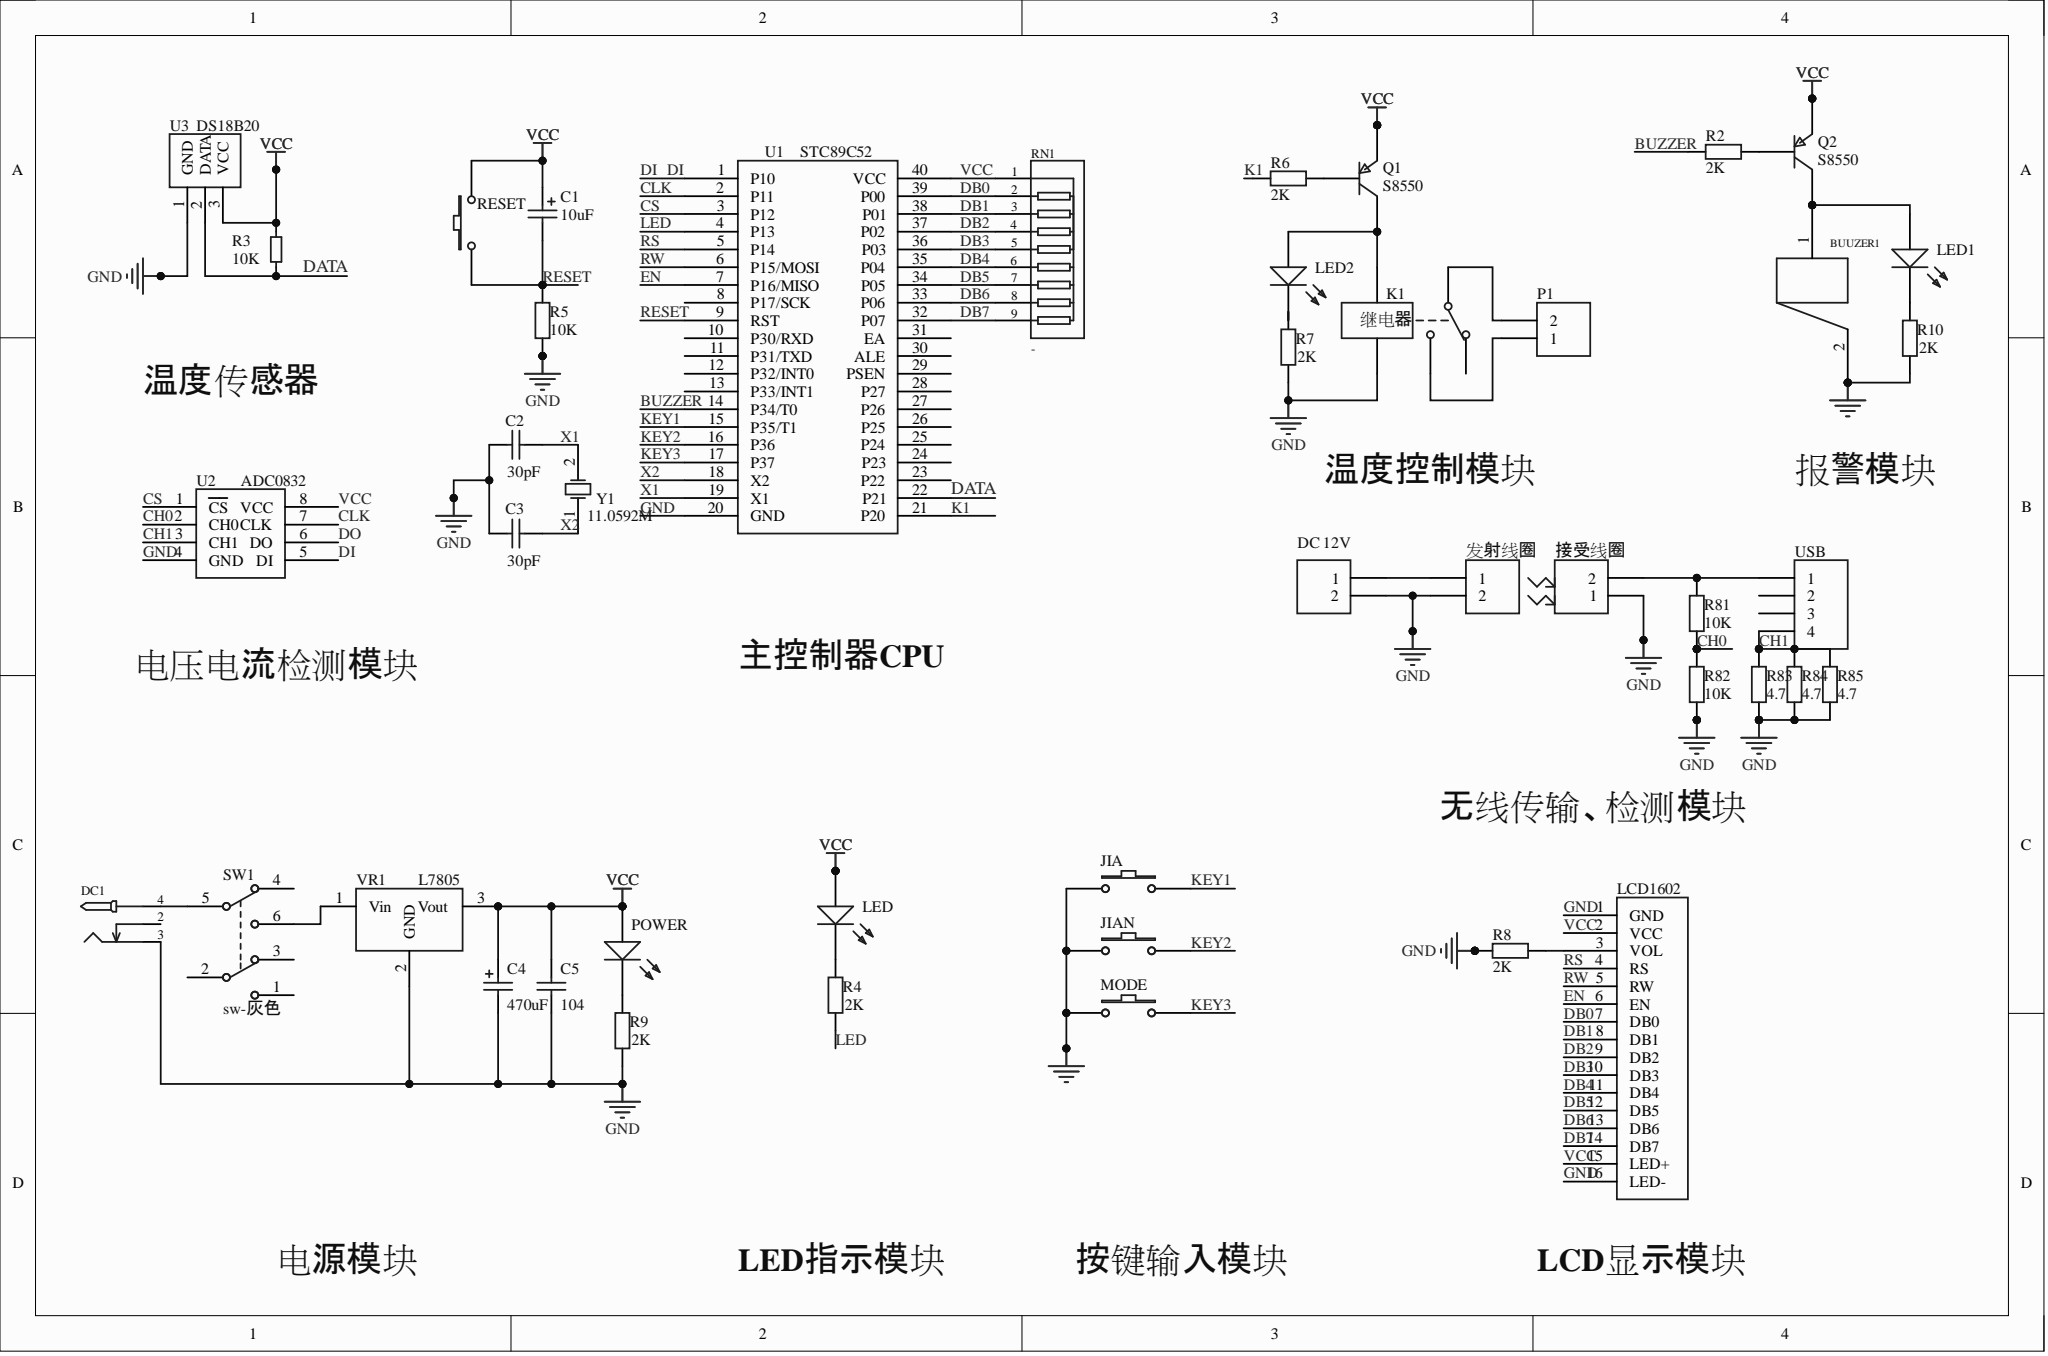Circuit board | Altium Designer | 45 parts | 43 nets
Bill of materials:
Comment,Description,Designator,Footprint,LibRef,Quantity
"BUZZER","","BUUZER1","BUZ-TH_BD12.0-P6.00-D0.9-RD","BUZZER","1"
"10uF","Polarized Capacitor (Axial)","C1","CAP-TH_BD5.0-P2.00-D0.8-FD-10UF50VC110GL","Cap Pol2","1"
"18pF","Capacitor","C2, C3","CAP-TH_L5.0-W2.5-P5.00-D1.0","Cap","2"
"470uF","Polarized Capacitor (Axial)","C4","CAP-TH_BD5.0-P2.00-D0.8-FD-10UF50VC110GL","Cap Pol2","1"
"104","Capacitor","C5","CAP-TH_L5.0-W2.5-P5.00-D1.0","Cap","1"
"","","DC1","DC-2.0","DC-005_2.0","1"
"Header 2","Header, 2-Pin","DC 12V, P1, 发射线圈, 接受线圈","HDR-TH_2P-P2.54-V-F","Header 2, Header 2_3, Header 2_1, Header 2_2","4"
"SW-PB","Switch","JIA, JIAN, MODE, RESET","KEY-TH_2P-L6.0-W3.9-P6.50","SW-PB_1, SW-PB_2, SW-PB_3, SW-PB","4"
"继电器","Single-Pole Dual-Throw Relay","K1","RELAY-TH_G2R-1_C9900014679","Relay-SPDT","1"
"LCD1602","","LCD1602","LCD1602","LCD1602","1"
"SI3317-H","Typical INFRARED GaAs LED","LED, LED1, LED2, POWER","LED_TH-3mm","LED0_1, LED0","4"
"S8550","PNP General Purpose Amplifier","Q1, Q2","TO-92-3_L4.6-W3.6-P1.27-L_1","2N3906","2"
"470","Resistor","R2, R4, R6, R7, R8, R9, R10, R81, R82, R83, R84, R85","Res_1/8W","0805, Res2, Res2_1","12"
"10K","[NoValue], Resistor","R3, R5","Res_1/8W","RES2","2"
"-","电阻器数:-;阻值:-;单个元件功率:-;","RN1","RES-ARRAY-TH_9P-P2.54-D1.0","排阻 10 K 5%","1"
"sw-灰色","","SW1","SW-TH_6P-L8.5-W8.5-P2.54","sw-灰色","1"
"STC89C52","","U1","DIP-40_L52.3-W13.9-P2.54-LS15.2-BL-BASE","AT89S52","1"
"ADC0832","","U2","DIP-8_L10.1-W6.3-P2.54-LS7.6-BL","Component_2","1"
"DS18B20","","U3","TO-92-3_L4.6-W3.6-P1.27-L_1","DS18B20","1"
"Header 4","Header, 4-Pin","USB","HDR-TH_4P-P2.54-V-F","Header 4","1"
"L7805","","VR1","TO-220AB-3_L10.4-W4.6-P2.54-L","78xx","1"
"11.059M","Crystal Oscillator","Y1","HC-49S_L11.0-W4.7-P4.88","XTAL","1"
Netlist (Protel format):
[
BUUZER1
BUZ-TH_BD12.0-P6.00-D0.9-RD
BUZZER



]
[
C1
CAP-TH_BD5.0-P2.00-D0.8-FD-10UF50VC110GL
10uF



]
[
C2
CAP-TH_L5.0-W2.5-P5.00-D1.0
18pF



]
[
C3
CAP-TH_L5.0-W2.5-P5.00-D1.0
18pF



]
[
C4
CAP-TH_BD5.0-P2.00-D0.8-FD-10UF50VC110GL
470uF



]
[
C5
CAP-TH_L5.0-W2.5-P5.00-D1.0
104



]
[
DC1
DC-2.0




]
[
DC 12V
HDR-TH_2P-P2.54-V-F
Header 2



]
[
JIA
KEY-TH_2P-L6.0-W3.9-P6.50
SW-PB



]
[
JIAN
KEY-TH_2P-L6.0-W3.9-P6.50
SW-PB



]
[
K1
RELAY-TH_G2R-1_C9900014679
继电器



]
[
LCD1602
LCD1602
LCD1602



]
[
LED
LED_TH-3mm
SI3317-H



]
[
LED1
LED_TH-3mm
SI3317-H



]
[
LED2
LED_TH-3mm
SI3317-H



]
[
MODE
KEY-TH_2P-L6.0-W3.9-P6.50
SW-PB



]
[
P1
HDR-TH_2P-P2.54-V-F
Header 2



]
[
POWER
LED_TH-3mm
SI3317-H



]
[
Q1
TO-92-3_L4.6-W3.6-P1.27-L_1
S8550



]
[
Q2
TO-92-3_L4.6-W3.6-P1.27-L_1
S8550



]
[
R2
Res_1/8W
470



]
[
R3
Res_1/8W
10K



]
[
R4
Res_1/8W
470



]
[
R5
Res_1/8W
10K



]
[
R6
Res_1/8W
470



]
[
R7
Res_1/8W
470



]
[
R8
Res_1/8W
470



]
[
R9
Res_1/8W
470



]
[
R10
Res_1/8W
470



]
[
R81
Res_1/8W
470



]
[
R82
Res_1/8W
470



]
[
R83
Res_1/8W
470



]
[
R84
Res_1/8W
470



]
[
R85
Res_1/8W
470



]
[
RESET
KEY-TH_2P-L6.0-W3.9-P6.50
SW-PB



]
[
RN1
RES-ARRAY-TH_9P-P2.54-D1.0
-



]
[
SW1
SW-TH_6P-L8.5-W8.5-P2.54
sw-灰色



]
[
U1
DIP-40_L52.3-W13.9-P2.54-LS15.2-BL-BASE
STC89C52



]
[
U2
DIP-8_L10.1-W6.3-P2.54-LS7.6-BL
ADC0832



]
[
U3
TO-92-3_L4.6-W3.6-P1.27-L_1
DS18B20



]
[
USB
HDR-TH_4P-P2.54-V-F
Header 4



]
[
VR1
TO-220AB-3_L10.4-W4.6-P2.54-L
L7805



]
[
Y1
HC-49S_L11.0-W4.7-P4.88
11.0592M



]
[
发射线圈
HDR-TH_2P-P2.54-V-F
Header 2



]
[
接受线圈
HDR-TH_2P-P2.54-V-F
Header 2



]
(
X2
C3-1
U1-18
Y1-1
)
(
X1
C2-1
U1-19
Y1-2
)
(
VCC
C1-2
C4-2
C5-2
LCD1602-2
LCD1602-15
LED-2
POWER-2
Q1-1
Q2-1
R3-2
RESET-2
RN1-1
U1-40
U2-8
U3-3
VR1-3
)
(
RW
LCD1602-5
U1-6
)
(
RS
LCD1602-4
U1-5
)
(
RESET
C1-1
R5-2
RESET-1
U1-9
)
(
NetSW1_6
SW1-6
VR1-1
)
(
NetR81_1
R81-1
USB-1
接受线圈-2
)
(
NetQ2_2
Q2-2
R2-1
)
(
NetQ1_2
Q1-2
R6-1
)
(
NetPOWER_1
POWER-1
R9-2
)
(
NetLED_1
LED-1
R4-2
)
(
NetLED2_1
LED2-1
R7-2
)
(
NetLED1_1
LED1-1
R10-2
)
(
NetLCD1602_3
LCD1602-3
R8-1
)
(
NetK1_4
K1-4
P1-2
)
(
NetK1_3
K1-3
P1-1
)
(
NetK1_1
K1-1
LED2-2
Q1-3
)
(
NetDC 12V_1
DC 12V-1
发射线圈-1
)
(
NetDC1_4
DC1-4
SW1-5
)
(
NetBUUZER1_1
BUUZER1-1
LED1-2
Q2-3
)
(
LED
R4-1
U1-4
)
(
KEY3
MODE-2
U1-17
)
(
KEY2
JIAN-2
U1-16
)
(
KEY1
JIA-2
U1-15
)
(
K1
R6-2
U1-21
)
(
GND
BUUZER1-2
C2-2
C3-2
C4-1
C5-1
DC1-3
DC 12V-2
JIA-1
JIAN-1
K1-5
LCD1602-1
LCD1602-16
MODE-1
R5-1
R7-1
R8-2
R9-1
R10-1
R82-2
R83-2
R84-2
R85-2
U1-20
U2-4
U3-1
VR1-2
发射线圈-2
接受线圈-1
)
(
EN
LCD1602-6
U1-7
)
(
DI
U1-1
U2-5
)
(
DB7
LCD1602-14
RN1-9
U1-32
)
(
DB6
LCD1602-13
RN1-8
U1-33
)
(
DB5
LCD1602-12
RN1-7
U1-34
)
(
DB4
LCD1602-11
RN1-6
U1-35
)
(
DB3
LCD1602-10
RN1-5
U1-36
)
(
DB2
LCD1602-9
RN1-4
U1-37
)
(
DB1
LCD1602-8
RN1-3
U1-38
)
(
DB0
LCD1602-7
RN1-2
U1-39
)
(
DATA
R3-1
U1-22
U3-2
)
(
CS
U1-3
U2-1
)
(
CLK
U1-2
U2-7
)
(
CH1
R83-1
R84-1
R85-1
U2-3
USB-4
)
(
CH0
R81-2
R82-1
U2-2
)
(
BUZZER
R2-2
U1-14
)